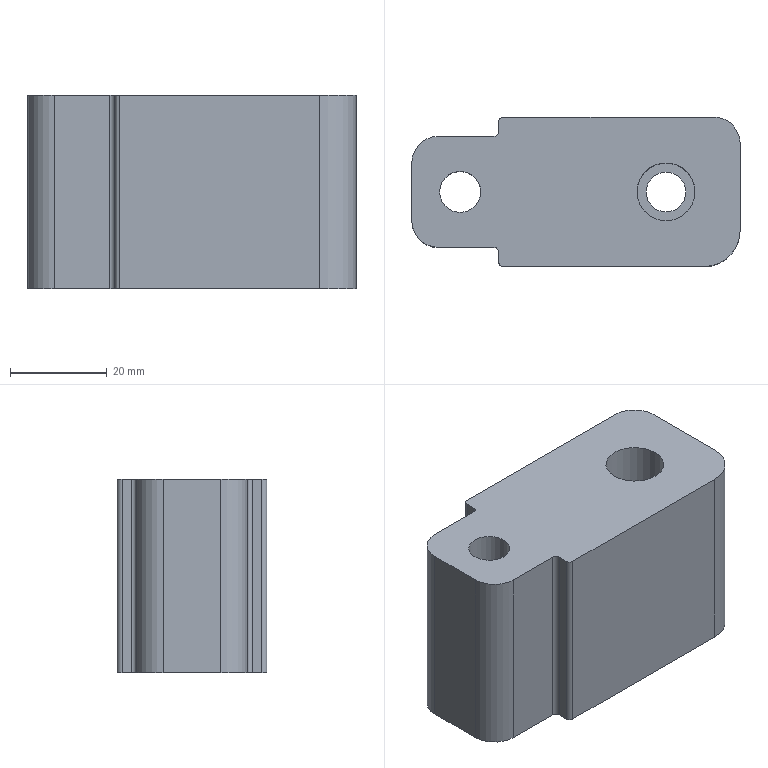Part | NX | features PS-2 2 | 1 solid | 24 faces | box 68 x 31 x 40 mm | volume 69968 mm3 | plane 12 | cylinder 12 | commonest cylinder face diameters 2 x4 11 x3 8.25 x1 8.5 x1 12 x1 14.5 x1
STEP:
#1=CARTESIAN_POINT('',(2363.049,-873.622,900.716));
#2=VERTEX_POINT('',#1);
#3=CARTESIAN_POINT('',(2404.549,-873.622,900.716));
#4=VERTEX_POINT('',#3);
#5=CARTESIAN_POINT('',(0.,-873.622,900.716));
#6=DIRECTION('',(1.,0.,0.));
#7=VECTOR('',#6,1000.);
#8=LINE('',#5,#7);
#9=EDGE_CURVE('',#2,#4,#8,.T.);
#10=ORIENTED_EDGE('',*,*,#9,.F.);
#11=CARTESIAN_POINT('',(2363.049,-873.622,860.716));
#12=VERTEX_POINT('',#11);
#13=CARTESIAN_POINT('',(2363.049,-873.622,830.716));
#14=DIRECTION('',(0.,0.,-1.));
#15=VECTOR('',#14,1000.);
#16=LINE('',#13,#15);
#17=EDGE_CURVE('',#2,#12,#16,.T.);
#18=ORIENTED_EDGE('',*,*,#17,.T.);
#19=CARTESIAN_POINT('',(2404.549,-873.622,860.716));
#20=VERTEX_POINT('',#19);
#21=CARTESIAN_POINT('',(2367.549,-873.622,860.716));
#22=DIRECTION('',(-1.,0.,0.));
#23=VECTOR('',#22,1000.);
#24=LINE('',#21,#23);
#25=EDGE_CURVE('',#20,#12,#24,.T.);
#26=ORIENTED_EDGE('',*,*,#25,.F.);
#27=CARTESIAN_POINT('',(2404.549,-873.622,830.716));
#28=DIRECTION('',(0.,0.,1.));
#29=VECTOR('',#28,1000.);
#30=LINE('',#27,#29);
#31=EDGE_CURVE('',#4,#20,#30,.F.);
#32=ORIENTED_EDGE('',*,*,#31,.F.);
#33=EDGE_LOOP('',(#10,#18,#26,#32));
#34=FACE_BOUND('',#33,.T.);
#35=CARTESIAN_POINT('',(2367.549,-873.622,830.716));
#36=DIRECTION('',(0.,-1.,0.));
#37=DIRECTION('',(0.,0.,-1.));
#38=AXIS2_PLACEMENT_3D('',#35,#36,#37);
#39=PLANE('',#38);
#40=ADVANCED_FACE('',(#34),#39,.T.);
#41=ORIENTED_EDGE('',*,*,#31,.T.);
#42=CARTESIAN_POINT('',(2412.049,-866.122,860.716));
#43=VERTEX_POINT('',#42);
#44=CARTESIAN_POINT('',(2404.549,-866.122,860.716));
#45=DIRECTION('',(0.,0.,1.));
#46=DIRECTION('',(1.,0.,0.));
#47=AXIS2_PLACEMENT_3D('',#44,#45,#46);
#48=CIRCLE('',#47,7.5);
#49=EDGE_CURVE('',#43,#20,#48,.F.);
#50=ORIENTED_EDGE('',*,*,#49,.F.);
#51=CARTESIAN_POINT('',(2412.049,-866.122,900.716));
#52=VERTEX_POINT('',#51);
#53=CARTESIAN_POINT('',(2412.049,-866.122,830.716));
#54=DIRECTION('',(0.,0.,-1.));
#55=VECTOR('',#54,1000.);
#56=LINE('',#53,#55);
#57=EDGE_CURVE('',#52,#43,#56,.T.);
#58=ORIENTED_EDGE('',*,*,#57,.F.);
#59=CARTESIAN_POINT('',(2404.549,-866.122,900.716));
#60=DIRECTION('',(0.,0.,1.));
#61=DIRECTION('',(1.,0.,0.));
#62=AXIS2_PLACEMENT_3D('',#59,#60,#61);
#63=CIRCLE('',#62,7.5);
#64=EDGE_CURVE('',#52,#4,#63,.F.);
#65=ORIENTED_EDGE('',*,*,#64,.T.);
#66=EDGE_LOOP('',(#41,#50,#58,#65));
#67=FACE_BOUND('',#66,.T.);
#68=CARTESIAN_POINT('',(2404.549,-866.122,830.716));
#69=DIRECTION('',(0.,0.,1.));
#70=DIRECTION('',(1.,0.,0.));
#71=AXIS2_PLACEMENT_3D('',#68,#69,#70);
#72=CYLINDRICAL_SURFACE('',#71,7.5);
#73=ADVANCED_FACE('',(#67),#72,.T.);
#74=ORIENTED_EDGE('',*,*,#57,.T.);
#75=CARTESIAN_POINT('',(2412.049,-848.122,860.716));
#76=VERTEX_POINT('',#75);
#77=CARTESIAN_POINT('',(2412.049,0.,860.716));
#78=DIRECTION('',(0.,1.,0.));
#79=VECTOR('',#78,1000.);
#80=LINE('',#77,#79);
#81=EDGE_CURVE('',#43,#76,#80,.T.);
#82=ORIENTED_EDGE('',*,*,#81,.T.);
#83=CARTESIAN_POINT('',(2412.049,-848.122,900.716));
#84=VERTEX_POINT('',#83);
#85=CARTESIAN_POINT('',(2412.049,-848.122,830.716));
#86=DIRECTION('',(0.,0.,1.));
#87=VECTOR('',#86,1000.);
#88=LINE('',#85,#87);
#89=EDGE_CURVE('',#84,#76,#88,.F.);
#90=ORIENTED_EDGE('',*,*,#89,.F.);
#91=CARTESIAN_POINT('',(2412.049,-866.122,900.716));
#92=DIRECTION('',(0.,-1.,0.));
#93=VECTOR('',#92,1000.);
#94=LINE('',#91,#93);
#95=EDGE_CURVE('',#84,#52,#94,.T.);
#96=ORIENTED_EDGE('',*,*,#95,.T.);
#97=EDGE_LOOP('',(#74,#82,#90,#96));
#98=FACE_BOUND('',#97,.T.);
#99=CARTESIAN_POINT('',(2412.049,-866.122,830.716));
#100=DIRECTION('',(1.,0.,0.));
#101=DIRECTION('',(0.,0.,-1.));
#102=AXIS2_PLACEMENT_3D('',#99,#100,#101);
#103=PLANE('',#102);
#104=ADVANCED_FACE('',(#98),#103,.T.);
#105=ORIENTED_EDGE('',*,*,#89,.T.);
#106=CARTESIAN_POINT('',(2406.549,-842.622,860.716));
#107=VERTEX_POINT('',#106);
#108=CARTESIAN_POINT('',(2406.549,-848.122,860.716));
#109=DIRECTION('',(0.,0.,1.));
#110=DIRECTION('',(1.,0.,0.));
#111=AXIS2_PLACEMENT_3D('',#108,#109,#110);
#112=CIRCLE('',#111,5.5);
#113=EDGE_CURVE('',#107,#76,#112,.F.);
#114=ORIENTED_EDGE('',*,*,#113,.F.);
#115=CARTESIAN_POINT('',(2406.549,-842.622,900.716));
#116=VERTEX_POINT('',#115);
#117=CARTESIAN_POINT('',(2406.549,-842.622,830.716));
#118=DIRECTION('',(0.,0.,1.));
#119=VECTOR('',#118,1000.);
#120=LINE('',#117,#119);
#121=EDGE_CURVE('',#116,#107,#120,.F.);
#122=ORIENTED_EDGE('',*,*,#121,.F.);
#123=CARTESIAN_POINT('',(2406.549,-848.122,900.716));
#124=DIRECTION('',(0.,0.,1.));
#125=DIRECTION('',(1.,0.,0.));
#126=AXIS2_PLACEMENT_3D('',#123,#124,#125);
#127=CIRCLE('',#126,5.5);
#128=EDGE_CURVE('',#84,#116,#127,.T.);
#129=ORIENTED_EDGE('',*,*,#128,.F.);
#130=EDGE_LOOP('',(#105,#114,#122,#129));
#131=FACE_BOUND('',#130,.T.);
#132=CARTESIAN_POINT('',(2406.549,-848.122,830.716));
#133=DIRECTION('',(0.,0.,1.));
#134=DIRECTION('',(1.,0.,0.));
#135=AXIS2_PLACEMENT_3D('',#132,#133,#134);
#136=CYLINDRICAL_SURFACE('',#135,5.5);
#137=ADVANCED_FACE('',(#131),#136,.T.);
#138=CARTESIAN_POINT('',(2363.049,-842.622,860.716));
#139=VERTEX_POINT('',#138);
#140=CARTESIAN_POINT('',(0.,-842.622,860.716));
#141=DIRECTION('',(-1.,0.,0.));
#142=VECTOR('',#141,1000.);
#143=LINE('',#140,#142);
#144=EDGE_CURVE('',#107,#139,#143,.T.);
#145=ORIENTED_EDGE('',*,*,#144,.T.);
#146=CARTESIAN_POINT('',(2363.049,-842.622,900.716));
#147=VERTEX_POINT('',#146);
#148=CARTESIAN_POINT('',(2363.049,-842.622,830.716));
#149=DIRECTION('',(0.,0.,1.));
#150=VECTOR('',#149,1000.);
#151=LINE('',#148,#150);
#152=EDGE_CURVE('',#139,#147,#151,.T.);
#153=ORIENTED_EDGE('',*,*,#152,.T.);
#154=CARTESIAN_POINT('',(2406.549,-842.622,900.716));
#155=DIRECTION('',(1.,0.,0.));
#156=VECTOR('',#155,1000.);
#157=LINE('',#154,#156);
#158=EDGE_CURVE('',#147,#116,#157,.T.);
#159=ORIENTED_EDGE('',*,*,#158,.T.);
#160=ORIENTED_EDGE('',*,*,#121,.T.);
#161=EDGE_LOOP('',(#145,#153,#159,#160));
#162=FACE_BOUND('',#161,.T.);
#163=CARTESIAN_POINT('',(2406.549,-842.622,830.716));
#164=DIRECTION('',(0.,1.,0.));
#165=DIRECTION('',(0.,0.,1.));
#166=AXIS2_PLACEMENT_3D('',#163,#164,#165);
#167=PLANE('',#166);
#168=ADVANCED_FACE('',(#162),#167,.T.);
#169=CARTESIAN_POINT('',(2362.049,-872.622,900.716));
#170=VERTEX_POINT('',#169);
#171=CARTESIAN_POINT('',(2362.049,-870.622,900.716));
#172=VERTEX_POINT('',#171);
#173=CARTESIAN_POINT('',(2362.049,-858.122,900.716));
#174=DIRECTION('',(0.,1.,0.));
#175=VECTOR('',#174,1000.);
#176=LINE('',#173,#175);
#177=EDGE_CURVE('',#170,#172,#176,.T.);
#178=ORIENTED_EDGE('',*,*,#177,.T.);
#179=CARTESIAN_POINT('',(2362.049,-870.622,860.716));
#180=VERTEX_POINT('',#179);
#181=CARTESIAN_POINT('',(2362.049,-870.622,860.716));
#182=DIRECTION('',(0.,0.,-1.));
#183=VECTOR('',#182,1000.);
#184=LINE('',#181,#183);
#185=EDGE_CURVE('',#172,#180,#184,.T.);
#186=ORIENTED_EDGE('',*,*,#185,.T.);
#187=CARTESIAN_POINT('',(2362.049,-872.622,860.716));
#188=VERTEX_POINT('',#187);
#189=CARTESIAN_POINT('',(2362.049,0.,860.716));
#190=DIRECTION('',(0.,-1.,0.));
#191=VECTOR('',#190,1000.);
#192=LINE('',#189,#191);
#193=EDGE_CURVE('',#180,#188,#192,.T.);
#194=ORIENTED_EDGE('',*,*,#193,.T.);
#195=CARTESIAN_POINT('',(2362.049,-872.622,875.716));
#196=DIRECTION('',(0.,0.,-1.));
#197=VECTOR('',#196,1000.);
#198=LINE('',#195,#197);
#199=EDGE_CURVE('',#188,#170,#198,.F.);
#200=ORIENTED_EDGE('',*,*,#199,.T.);
#201=EDGE_LOOP('',(#178,#186,#194,#200));
#202=FACE_BOUND('',#201,.T.);
#203=CARTESIAN_POINT('',(2362.049,-858.122,875.716));
#204=DIRECTION('',(-1.,0.,0.));
#205=DIRECTION('',(0.,0.,1.));
#206=AXIS2_PLACEMENT_3D('',#203,#204,#205);
#207=PLANE('',#206);
#208=ADVANCED_FACE('',(#202),#207,.T.);
#209=CARTESIAN_POINT('',(2362.049,-845.622,900.716));
#210=VERTEX_POINT('',#209);
#211=CARTESIAN_POINT('',(2362.049,-843.622,900.716));
#212=VERTEX_POINT('',#211);
#213=CARTESIAN_POINT('',(2362.049,-858.122,900.716));
#214=DIRECTION('',(0.,1.,0.));
#215=VECTOR('',#214,1000.);
#216=LINE('',#213,#215);
#217=EDGE_CURVE('',#210,#212,#216,.T.);
#218=ORIENTED_EDGE('',*,*,#217,.T.);
#219=CARTESIAN_POINT('',(2362.049,-843.622,860.716));
#220=VERTEX_POINT('',#219);
#221=CARTESIAN_POINT('',(2362.049,-843.622,875.716));
#222=DIRECTION('',(0.,0.,1.));
#223=VECTOR('',#222,1000.);
#224=LINE('',#221,#223);
#225=EDGE_CURVE('',#212,#220,#224,.F.);
#226=ORIENTED_EDGE('',*,*,#225,.T.);
#227=CARTESIAN_POINT('',(2362.049,-845.622,860.716));
#228=VERTEX_POINT('',#227);
#229=CARTESIAN_POINT('',(2362.049,0.,860.716));
#230=DIRECTION('',(0.,-1.,0.));
#231=VECTOR('',#230,1000.);
#232=LINE('',#229,#231);
#233=EDGE_CURVE('',#220,#228,#232,.T.);
#234=ORIENTED_EDGE('',*,*,#233,.T.);
#235=CARTESIAN_POINT('',(2362.049,-845.622,890.716));
#236=DIRECTION('',(0.,0.,1.));
#237=VECTOR('',#236,1000.);
#238=LINE('',#235,#237);
#239=EDGE_CURVE('',#228,#210,#238,.T.);
#240=ORIENTED_EDGE('',*,*,#239,.T.);
#241=EDGE_LOOP('',(#218,#226,#234,#240));
#242=FACE_BOUND('',#241,.T.);
#243=CARTESIAN_POINT('',(2362.049,-858.122,875.716));
#244=DIRECTION('',(-1.,0.,0.));
#245=DIRECTION('',(0.,0.,1.));
#246=AXIS2_PLACEMENT_3D('',#243,#244,#245);
#247=PLANE('',#246);
#248=ADVANCED_FACE('',(#242),#247,.T.);
#249=CARTESIAN_POINT('',(2344.049,-852.122,900.716));
#250=VERTEX_POINT('',#249);
#251=CARTESIAN_POINT('',(2344.049,-852.122,860.716));
#252=VERTEX_POINT('',#251);
#253=CARTESIAN_POINT('',(2344.049,-852.122,830.716));
#254=DIRECTION('',(0.,0.,1.));
#255=VECTOR('',#254,1000.);
#256=LINE('',#253,#255);
#257=EDGE_CURVE('',#250,#252,#256,.F.);
#258=ORIENTED_EDGE('',*,*,#257,.T.);
#259=CARTESIAN_POINT('',(2344.049,-864.122,860.716));
#260=VERTEX_POINT('',#259);
#261=CARTESIAN_POINT('',(2344.049,-848.122,860.716));
#262=DIRECTION('',(0.,1.,0.));
#263=VECTOR('',#262,1000.);
#264=LINE('',#261,#263);
#265=EDGE_CURVE('',#260,#252,#264,.T.);
#266=ORIENTED_EDGE('',*,*,#265,.F.);
#267=CARTESIAN_POINT('',(2344.049,-864.122,900.716));
#268=VERTEX_POINT('',#267);
#269=CARTESIAN_POINT('',(2344.049,-864.122,830.716));
#270=DIRECTION('',(0.,0.,1.));
#271=VECTOR('',#270,1000.);
#272=LINE('',#269,#271);
#273=EDGE_CURVE('',#268,#260,#272,.F.);
#274=ORIENTED_EDGE('',*,*,#273,.F.);
#275=CARTESIAN_POINT('',(2344.049,-848.122,900.716));
#276=DIRECTION('',(0.,1.,0.));
#277=VECTOR('',#276,1000.);
#278=LINE('',#275,#277);
#279=EDGE_CURVE('',#268,#250,#278,.T.);
#280=ORIENTED_EDGE('',*,*,#279,.T.);
#281=EDGE_LOOP('',(#258,#266,#274,#280));
#282=FACE_BOUND('',#281,.T.);
#283=CARTESIAN_POINT('',(2344.049,-848.122,830.716));
#284=DIRECTION('',(-1.,0.,0.));
#285=DIRECTION('',(0.,0.,1.));
#286=AXIS2_PLACEMENT_3D('',#283,#284,#285);
#287=PLANE('',#286);
#288=ADVANCED_FACE('',(#282),#287,.T.);
#289=ORIENTED_EDGE('',*,*,#273,.T.);
#290=CARTESIAN_POINT('',(2349.549,-869.622,860.716));
#291=VERTEX_POINT('',#290);
#292=CARTESIAN_POINT('',(2349.549,-864.122,860.716));
#293=DIRECTION('',(0.,0.,1.));
#294=DIRECTION('',(1.,0.,0.));
#295=AXIS2_PLACEMENT_3D('',#292,#293,#294);
#296=CIRCLE('',#295,5.5);
#297=EDGE_CURVE('',#291,#260,#296,.F.);
#298=ORIENTED_EDGE('',*,*,#297,.F.);
#299=CARTESIAN_POINT('',(2349.549,-869.622,900.716));
#300=VERTEX_POINT('',#299);
#301=CARTESIAN_POINT('',(2349.549,-869.622,830.716));
#302=DIRECTION('',(0.,0.,-1.));
#303=VECTOR('',#302,1000.);
#304=LINE('',#301,#303);
#305=EDGE_CURVE('',#300,#291,#304,.T.);
#306=ORIENTED_EDGE('',*,*,#305,.F.);
#307=CARTESIAN_POINT('',(2349.549,-864.122,900.716));
#308=DIRECTION('',(0.,0.,1.));
#309=DIRECTION('',(1.,0.,0.));
#310=AXIS2_PLACEMENT_3D('',#307,#308,#309);
#311=CIRCLE('',#310,5.5);
#312=EDGE_CURVE('',#300,#268,#311,.F.);
#313=ORIENTED_EDGE('',*,*,#312,.T.);
#314=EDGE_LOOP('',(#289,#298,#306,#313));
#315=FACE_BOUND('',#314,.T.);
#316=CARTESIAN_POINT('',(2349.549,-864.122,830.716));
#317=DIRECTION('',(0.,0.,1.));
#318=DIRECTION('',(1.,0.,0.));
#319=AXIS2_PLACEMENT_3D('',#316,#317,#318);
#320=CYLINDRICAL_SURFACE('',#319,5.5);
#321=ADVANCED_FACE('',(#315),#320,.T.);
#322=CARTESIAN_POINT('',(2361.049,-869.622,860.716));
#323=VERTEX_POINT('',#322);
#324=CARTESIAN_POINT('',(2367.549,-869.622,860.716));
#325=DIRECTION('',(-1.,0.,0.));
#326=VECTOR('',#325,1000.);
#327=LINE('',#324,#326);
#328=EDGE_CURVE('',#323,#291,#327,.T.);
#329=ORIENTED_EDGE('',*,*,#328,.F.);
#330=CARTESIAN_POINT('',(2361.049,-869.622,900.716));
#331=VERTEX_POINT('',#330);
#332=CARTESIAN_POINT('',(2361.049,-869.622,890.716));
#333=DIRECTION('',(0.,0.,-1.));
#334=VECTOR('',#333,1000.);
#335=LINE('',#332,#334);
#336=EDGE_CURVE('',#323,#331,#335,.F.);
#337=ORIENTED_EDGE('',*,*,#336,.T.);
#338=CARTESIAN_POINT('',(0.,-869.622,900.716));
#339=DIRECTION('',(1.,0.,0.));
#340=VECTOR('',#339,1000.);
#341=LINE('',#338,#340);
#342=EDGE_CURVE('',#300,#331,#341,.T.);
#343=ORIENTED_EDGE('',*,*,#342,.F.);
#344=ORIENTED_EDGE('',*,*,#305,.T.);
#345=EDGE_LOOP('',(#329,#337,#343,#344));
#346=FACE_BOUND('',#345,.T.);
#347=CARTESIAN_POINT('',(2367.549,-869.622,830.716));
#348=DIRECTION('',(0.,-1.,0.));
#349=DIRECTION('',(0.,0.,-1.));
#350=AXIS2_PLACEMENT_3D('',#347,#348,#349);
#351=PLANE('',#350);
#352=ADVANCED_FACE('',(#346),#351,.T.);
#353=CARTESIAN_POINT('',(2349.549,-846.622,900.716));
#354=VERTEX_POINT('',#353);
#355=CARTESIAN_POINT('',(2361.049,-846.622,900.716));
#356=VERTEX_POINT('',#355);
#357=CARTESIAN_POINT('',(2406.549,-846.622,900.716));
#358=DIRECTION('',(1.,0.,0.));
#359=VECTOR('',#358,1000.);
#360=LINE('',#357,#359);
#361=EDGE_CURVE('',#354,#356,#360,.T.);
#362=ORIENTED_EDGE('',*,*,#361,.T.);
#363=CARTESIAN_POINT('',(2361.049,-846.622,860.716));
#364=VERTEX_POINT('',#363);
#365=CARTESIAN_POINT('',(2361.049,-846.622,860.716));
#366=DIRECTION('',(0.,0.,1.));
#367=VECTOR('',#366,1000.);
#368=LINE('',#365,#367);
#369=EDGE_CURVE('',#356,#364,#368,.F.);
#370=ORIENTED_EDGE('',*,*,#369,.T.);
#371=CARTESIAN_POINT('',(2349.549,-846.622,860.716));
#372=VERTEX_POINT('',#371);
#373=CARTESIAN_POINT('',(0.,-846.622,860.716));
#374=DIRECTION('',(-1.,0.,0.));
#375=VECTOR('',#374,1000.);
#376=LINE('',#373,#375);
#377=EDGE_CURVE('',#364,#372,#376,.T.);
#378=ORIENTED_EDGE('',*,*,#377,.T.);
#379=CARTESIAN_POINT('',(2349.549,-846.622,830.716));
#380=DIRECTION('',(0.,0.,1.));
#381=VECTOR('',#380,1000.);
#382=LINE('',#379,#381);
#383=EDGE_CURVE('',#354,#372,#382,.F.);
#384=ORIENTED_EDGE('',*,*,#383,.F.);
#385=EDGE_LOOP('',(#362,#370,#378,#384));
#386=FACE_BOUND('',#385,.T.);
#387=CARTESIAN_POINT('',(2406.549,-846.622,830.716));
#388=DIRECTION('',(0.,1.,0.));
#389=DIRECTION('',(0.,0.,1.));
#390=AXIS2_PLACEMENT_3D('',#387,#388,#389);
#391=PLANE('',#390);
#392=ADVANCED_FACE('',(#386),#391,.T.);
#393=ORIENTED_EDGE('',*,*,#383,.T.);
#394=CARTESIAN_POINT('',(2349.549,-852.122,860.716));
#395=DIRECTION('',(0.,0.,1.));
#396=DIRECTION('',(1.,0.,0.));
#397=AXIS2_PLACEMENT_3D('',#394,#395,#396);
#398=CIRCLE('',#397,5.5);
#399=EDGE_CURVE('',#372,#252,#398,.T.);
#400=ORIENTED_EDGE('',*,*,#399,.T.);
#401=ORIENTED_EDGE('',*,*,#257,.F.);
#402=CARTESIAN_POINT('',(2349.549,-852.122,900.716));
#403=DIRECTION('',(0.,0.,1.));
#404=DIRECTION('',(1.,0.,0.));
#405=AXIS2_PLACEMENT_3D('',#402,#403,#404);
#406=CIRCLE('',#405,5.5);
#407=EDGE_CURVE('',#354,#250,#406,.T.);
#408=ORIENTED_EDGE('',*,*,#407,.F.);
#409=EDGE_LOOP('',(#393,#400,#401,#408));
#410=FACE_BOUND('',#409,.T.);
#411=CARTESIAN_POINT('',(2349.549,-852.122,830.716));
#412=DIRECTION('',(0.,0.,1.));
#413=DIRECTION('',(1.,0.,0.));
#414=AXIS2_PLACEMENT_3D('',#411,#412,#413);
#415=CYLINDRICAL_SURFACE('',#414,5.5);
#416=ADVANCED_FACE('',(#410),#415,.T.);
#417=CARTESIAN_POINT('',(2400.824,-858.122,860.716));
#418=VERTEX_POINT('',#417);
#419=CARTESIAN_POINT('',(2396.699,-858.122,860.716));
#420=DIRECTION('',(0.,0.,1.));
#421=DIRECTION('',(1.,0.,0.));
#422=AXIS2_PLACEMENT_3D('',#419,#420,#421);
#423=CIRCLE('',#422,4.125);
#424=EDGE_CURVE('',#418,#418,#423,.T.);
#425=ORIENTED_EDGE('',*,*,#424,.T.);
#426=EDGE_LOOP('',(#425));
#427=FACE_BOUND('',#426,.T.);
#428=CARTESIAN_POINT('',(2361.299,-858.122,860.716));
#429=VERTEX_POINT('',#428);
#430=CARTESIAN_POINT('',(2354.049,-858.122,860.716));
#431=DIRECTION('',(0.,0.,1.));
#432=DIRECTION('',(1.,0.,0.));
#433=AXIS2_PLACEMENT_3D('',#430,#431,#432);
#434=CIRCLE('',#433,7.25);
#435=EDGE_CURVE('',#429,#429,#434,.T.);
#436=ORIENTED_EDGE('',*,*,#435,.T.);
#437=EDGE_LOOP('',(#436));
#438=FACE_BOUND('',#437,.T.);
#439=ORIENTED_EDGE('',*,*,#233,.F.);
#440=CARTESIAN_POINT('',(2363.049,-843.622,860.716));
#441=DIRECTION('',(0.,0.,1.));
#442=DIRECTION('',(1.,0.,0.));
#443=AXIS2_PLACEMENT_3D('',#440,#441,#442);
#444=CIRCLE('',#443,1.);
#445=EDGE_CURVE('',#220,#139,#444,.F.);
#446=ORIENTED_EDGE('',*,*,#445,.T.);
#447=ORIENTED_EDGE('',*,*,#144,.F.);
#448=ORIENTED_EDGE('',*,*,#113,.T.);
#449=ORIENTED_EDGE('',*,*,#81,.F.);
#450=ORIENTED_EDGE('',*,*,#49,.T.);
#451=ORIENTED_EDGE('',*,*,#25,.T.);
#452=CARTESIAN_POINT('',(2363.049,-872.622,860.716));
#453=DIRECTION('',(0.,0.,1.));
#454=DIRECTION('',(1.,0.,0.));
#455=AXIS2_PLACEMENT_3D('',#452,#453,#454);
#456=CIRCLE('',#455,1.);
#457=EDGE_CURVE('',#12,#188,#456,.F.);
#458=ORIENTED_EDGE('',*,*,#457,.T.);
#459=ORIENTED_EDGE('',*,*,#193,.F.);
#460=CARTESIAN_POINT('',(2361.049,-870.622,860.716));
#461=DIRECTION('',(0.,0.,1.));
#462=DIRECTION('',(1.,0.,0.));
#463=AXIS2_PLACEMENT_3D('',#460,#461,#462);
#464=CIRCLE('',#463,1.);
#465=EDGE_CURVE('',#180,#323,#464,.T.);
#466=ORIENTED_EDGE('',*,*,#465,.T.);
#467=ORIENTED_EDGE('',*,*,#328,.T.);
#468=ORIENTED_EDGE('',*,*,#297,.T.);
#469=ORIENTED_EDGE('',*,*,#265,.T.);
#470=ORIENTED_EDGE('',*,*,#399,.F.);
#471=ORIENTED_EDGE('',*,*,#377,.F.);
#472=CARTESIAN_POINT('',(2361.049,-845.622,860.716));
#473=DIRECTION('',(0.,0.,1.));
#474=DIRECTION('',(1.,0.,0.));
#475=AXIS2_PLACEMENT_3D('',#472,#473,#474);
#476=CIRCLE('',#475,1.);
#477=EDGE_CURVE('',#364,#228,#476,.T.);
#478=ORIENTED_EDGE('',*,*,#477,.T.);
#479=EDGE_LOOP('',(#439,#446,#447,#448,#449,#450,#451,#458,#459,#466,#467,#468,#469,#470,#471,#478));
#480=FACE_BOUND('',#479,.T.);
#481=CARTESIAN_POINT('',(0.,0.,860.716));
#482=DIRECTION('',(0.,0.,1.));
#483=DIRECTION('',(1.,0.,0.));
#484=AXIS2_PLACEMENT_3D('',#481,#482,#483);
#485=PLANE('',#484);
#486=ADVANCED_FACE('',(#427,#438,#480),#485,.F.);
#487=CARTESIAN_POINT('',(2402.699,-858.122,900.716));
#488=VERTEX_POINT('',#487);
#489=CARTESIAN_POINT('',(2396.699,-858.122,900.716));
#490=DIRECTION('',(0.,0.,1.));
#491=DIRECTION('',(1.,0.,0.));
#492=AXIS2_PLACEMENT_3D('',#489,#490,#491);
#493=CIRCLE('',#492,6.);
#494=EDGE_CURVE('',#488,#488,#493,.T.);
#495=ORIENTED_EDGE('',*,*,#494,.F.);
#496=EDGE_LOOP('',(#495));
#497=FACE_BOUND('',#496,.T.);
#498=CARTESIAN_POINT('',(2358.299,-858.122,900.716));
#499=VERTEX_POINT('',#498);
#500=CARTESIAN_POINT('',(2354.049,-858.122,900.716));
#501=DIRECTION('',(0.,0.,1.));
#502=DIRECTION('',(1.,0.,0.));
#503=AXIS2_PLACEMENT_3D('',#500,#501,#502);
#504=CIRCLE('',#503,4.25);
#505=EDGE_CURVE('',#499,#499,#504,.T.);
#506=ORIENTED_EDGE('',*,*,#505,.F.);
#507=EDGE_LOOP('',(#506));
#508=FACE_BOUND('',#507,.T.);
#509=ORIENTED_EDGE('',*,*,#158,.F.);
#510=CARTESIAN_POINT('',(2363.049,-843.622,900.716));
#511=DIRECTION('',(0.,0.,1.));
#512=DIRECTION('',(1.,0.,0.));
#513=AXIS2_PLACEMENT_3D('',#510,#511,#512);
#514=CIRCLE('',#513,1.);
#515=EDGE_CURVE('',#147,#212,#514,.T.);
#516=ORIENTED_EDGE('',*,*,#515,.T.);
#517=ORIENTED_EDGE('',*,*,#217,.F.);
#518=CARTESIAN_POINT('',(2361.049,-845.622,900.716));
#519=DIRECTION('',(0.,0.,1.));
#520=DIRECTION('',(1.,0.,0.));
#521=AXIS2_PLACEMENT_3D('',#518,#519,#520);
#522=CIRCLE('',#521,1.);
#523=EDGE_CURVE('',#210,#356,#522,.F.);
#524=ORIENTED_EDGE('',*,*,#523,.T.);
#525=ORIENTED_EDGE('',*,*,#361,.F.);
#526=ORIENTED_EDGE('',*,*,#407,.T.);
#527=ORIENTED_EDGE('',*,*,#279,.F.);
#528=ORIENTED_EDGE('',*,*,#312,.F.);
#529=ORIENTED_EDGE('',*,*,#342,.T.);
#530=CARTESIAN_POINT('',(2361.049,-870.622,900.716));
#531=DIRECTION('',(0.,0.,1.));
#532=DIRECTION('',(1.,0.,0.));
#533=AXIS2_PLACEMENT_3D('',#530,#531,#532);
#534=CIRCLE('',#533,1.);
#535=EDGE_CURVE('',#331,#172,#534,.F.);
#536=ORIENTED_EDGE('',*,*,#535,.T.);
#537=ORIENTED_EDGE('',*,*,#177,.F.);
#538=CARTESIAN_POINT('',(2363.049,-872.622,900.716));
#539=DIRECTION('',(0.,0.,1.));
#540=DIRECTION('',(1.,0.,0.));
#541=AXIS2_PLACEMENT_3D('',#538,#539,#540);
#542=CIRCLE('',#541,1.);
#543=EDGE_CURVE('',#170,#2,#542,.T.);
#544=ORIENTED_EDGE('',*,*,#543,.T.);
#545=ORIENTED_EDGE('',*,*,#9,.T.);
#546=ORIENTED_EDGE('',*,*,#64,.F.);
#547=ORIENTED_EDGE('',*,*,#95,.F.);
#548=ORIENTED_EDGE('',*,*,#128,.T.);
#549=EDGE_LOOP('',(#509,#516,#517,#524,#525,#526,#527,#528,#529,#536,#537,#544,#545,#546,#547,#548));
#550=FACE_BOUND('',#549,.T.);
#551=CARTESIAN_POINT('',(0.,0.,900.716));
#552=DIRECTION('',(0.,0.,1.));
#553=DIRECTION('',(1.,0.,0.));
#554=AXIS2_PLACEMENT_3D('',#551,#552,#553);
#555=PLANE('',#554);
#556=ADVANCED_FACE('',(#497,#508,#550),#555,.T.);
#557=CARTESIAN_POINT('',(2354.049,-850.872,871.716));
#558=VERTEX_POINT('',#557);
#559=CARTESIAN_POINT('',(2354.049,-858.122,871.716));
#560=DIRECTION('',(0.,0.,-1.));
#561=DIRECTION('',(0.,1.,0.));
#562=AXIS2_PLACEMENT_3D('',#559,#560,#561);
#563=CIRCLE('',#562,7.25);
#564=EDGE_CURVE('',#558,#558,#563,.F.);
#565=ORIENTED_EDGE('',*,*,#564,.T.);
#566=EDGE_LOOP('',(#565));
#567=FACE_BOUND('',#566,.T.);
#568=ORIENTED_EDGE('',*,*,#435,.F.);
#569=EDGE_LOOP('',(#568));
#570=FACE_BOUND('',#569,.T.);
#571=CARTESIAN_POINT('',(2354.049,-858.122,871.716));
#572=DIRECTION('',(0.,0.,-1.));
#573=DIRECTION('',(-1.,0.,0.));
#574=AXIS2_PLACEMENT_3D('',#571,#572,#573);
#575=CYLINDRICAL_SURFACE('',#574,7.25);
#576=ADVANCED_FACE('',(#567,#570),#575,.F.);
#577=ORIENTED_EDGE('',*,*,#505,.T.);
#578=EDGE_LOOP('',(#577));
#579=FACE_BOUND('',#578,.T.);
#580=CARTESIAN_POINT('',(2349.799,-858.122,871.716));
#581=VERTEX_POINT('',#580);
#582=CARTESIAN_POINT('',(2354.049,-858.122,871.716));
#583=DIRECTION('',(0.,0.,-1.));
#584=DIRECTION('',(-1.,0.,0.));
#585=AXIS2_PLACEMENT_3D('',#582,#583,#584);
#586=CIRCLE('',#585,4.25);
#587=EDGE_CURVE('',#581,#581,#586,.T.);
#588=ORIENTED_EDGE('',*,*,#587,.T.);
#589=EDGE_LOOP('',(#588));
#590=FACE_BOUND('',#589,.T.);
#591=CARTESIAN_POINT('',(2354.049,-858.122,891.716));
#592=DIRECTION('',(0.,0.,-1.));
#593=DIRECTION('',(-1.,0.,0.));
#594=AXIS2_PLACEMENT_3D('',#591,#592,#593);
#595=CYLINDRICAL_SURFACE('',#594,4.25);
#596=ADVANCED_FACE('',(#579,#590),#595,.F.);
#597=ORIENTED_EDGE('',*,*,#587,.F.);
#598=EDGE_LOOP('',(#597));
#599=FACE_BOUND('',#598,.T.);
#600=ORIENTED_EDGE('',*,*,#564,.F.);
#601=EDGE_LOOP('',(#600));
#602=FACE_BOUND('',#601,.T.);
#603=CARTESIAN_POINT('',(2354.049,-858.122,871.716));
#604=DIRECTION('',(0.,0.,-1.));
#605=DIRECTION('',(-1.,0.,0.));
#606=AXIS2_PLACEMENT_3D('',#603,#604,#605);
#607=PLANE('',#606);
#608=ADVANCED_FACE('',(#599,#602),#607,.T.);
#609=ORIENTED_EDGE('',*,*,#445,.F.);
#610=ORIENTED_EDGE('',*,*,#225,.F.);
#611=ORIENTED_EDGE('',*,*,#515,.F.);
#612=ORIENTED_EDGE('',*,*,#152,.F.);
#613=EDGE_LOOP('',(#609,#610,#611,#612));
#614=FACE_BOUND('',#613,.T.);
#615=CARTESIAN_POINT('',(2363.049,-843.622,830.716));
#616=DIRECTION('',(0.,0.,1.));
#617=DIRECTION('',(1.,0.,0.));
#618=AXIS2_PLACEMENT_3D('',#615,#616,#617);
#619=CYLINDRICAL_SURFACE('',#618,1.);
#620=ADVANCED_FACE('',(#614),#619,.T.);
#621=ORIENTED_EDGE('',*,*,#477,.F.);
#622=ORIENTED_EDGE('',*,*,#369,.F.);
#623=ORIENTED_EDGE('',*,*,#523,.F.);
#624=ORIENTED_EDGE('',*,*,#239,.F.);
#625=EDGE_LOOP('',(#621,#622,#623,#624));
#626=FACE_BOUND('',#625,.T.);
#627=CARTESIAN_POINT('',(2361.049,-845.622,875.716));
#628=DIRECTION('',(0.,0.,-1.));
#629=DIRECTION('',(-1.,0.,0.));
#630=AXIS2_PLACEMENT_3D('',#627,#628,#629);
#631=CYLINDRICAL_SURFACE('',#630,1.);
#632=ADVANCED_FACE('',(#626),#631,.F.);
#633=ORIENTED_EDGE('',*,*,#535,.F.);
#634=ORIENTED_EDGE('',*,*,#336,.F.);
#635=ORIENTED_EDGE('',*,*,#465,.F.);
#636=ORIENTED_EDGE('',*,*,#185,.F.);
#637=EDGE_LOOP('',(#633,#634,#635,#636));
#638=FACE_BOUND('',#637,.T.);
#639=CARTESIAN_POINT('',(2361.049,-870.622,875.716));
#640=DIRECTION('',(0.,0.,1.));
#641=DIRECTION('',(1.,0.,0.));
#642=AXIS2_PLACEMENT_3D('',#639,#640,#641);
#643=CYLINDRICAL_SURFACE('',#642,1.);
#644=ADVANCED_FACE('',(#638),#643,.F.);
#645=ORIENTED_EDGE('',*,*,#543,.F.);
#646=ORIENTED_EDGE('',*,*,#199,.F.);
#647=ORIENTED_EDGE('',*,*,#457,.F.);
#648=ORIENTED_EDGE('',*,*,#17,.F.);
#649=EDGE_LOOP('',(#645,#646,#647,#648));
#650=FACE_BOUND('',#649,.T.);
#651=CARTESIAN_POINT('',(2363.049,-872.622,830.716));
#652=DIRECTION('',(0.,0.,-1.));
#653=DIRECTION('',(-1.,0.,0.));
#654=AXIS2_PLACEMENT_3D('',#651,#652,#653);
#655=CYLINDRICAL_SURFACE('',#654,1.);
#656=ADVANCED_FACE('',(#650),#655,.T.);
#657=CARTESIAN_POINT('',(2392.574,-858.122,871.716));
#658=VERTEX_POINT('',#657);
#659=CARTESIAN_POINT('',(2396.699,-858.122,871.716));
#660=DIRECTION('',(0.,0.,-1.));
#661=DIRECTION('',(-1.,0.,0.));
#662=AXIS2_PLACEMENT_3D('',#659,#660,#661);
#663=CIRCLE('',#662,4.125);
#664=EDGE_CURVE('',#658,#658,#663,.T.);
#665=ORIENTED_EDGE('',*,*,#664,.F.);
#666=EDGE_LOOP('',(#665));
#667=FACE_BOUND('',#666,.T.);
#668=ORIENTED_EDGE('',*,*,#424,.F.);
#669=EDGE_LOOP('',(#668));
#670=FACE_BOUND('',#669,.T.);
#671=CARTESIAN_POINT('',(2396.699,-858.122,935.716));
#672=DIRECTION('',(0.,0.,-1.));
#673=DIRECTION('',(1.,0.,0.));
#674=AXIS2_PLACEMENT_3D('',#671,#672,#673);
#675=CYLINDRICAL_SURFACE('',#674,4.125);
#676=ADVANCED_FACE('',(#667,#670),#675,.F.);
#677=ORIENTED_EDGE('',*,*,#664,.T.);
#678=EDGE_LOOP('',(#677));
#679=FACE_BOUND('',#678,.T.);
#680=CARTESIAN_POINT('',(2402.699,-858.122,871.716));
#681=VERTEX_POINT('',#680);
#682=CARTESIAN_POINT('',(2396.699,-858.122,871.716));
#683=DIRECTION('',(0.,0.,1.));
#684=DIRECTION('',(1.,0.,0.));
#685=AXIS2_PLACEMENT_3D('',#682,#683,#684);
#686=CIRCLE('',#685,6.);
#687=EDGE_CURVE('',#681,#681,#686,.F.);
#688=ORIENTED_EDGE('',*,*,#687,.F.);
#689=EDGE_LOOP('',(#688));
#690=FACE_BOUND('',#689,.T.);
#691=CARTESIAN_POINT('',(2396.699,-858.122,871.716));
#692=DIRECTION('',(0.,0.,-1.));
#693=DIRECTION('',(-1.,0.,0.));
#694=AXIS2_PLACEMENT_3D('',#691,#692,#693);
#695=PLANE('',#694);
#696=ADVANCED_FACE('',(#679,#690),#695,.F.);
#697=ORIENTED_EDGE('',*,*,#494,.T.);
#698=EDGE_LOOP('',(#697));
#699=FACE_BOUND('',#698,.T.);
#700=ORIENTED_EDGE('',*,*,#687,.T.);
#701=EDGE_LOOP('',(#700));
#702=FACE_BOUND('',#701,.T.);
#703=CARTESIAN_POINT('',(2396.699,-858.122,935.716));
#704=DIRECTION('',(0.,0.,-1.));
#705=DIRECTION('',(1.,0.,0.));
#706=AXIS2_PLACEMENT_3D('',#703,#704,#705);
#707=CYLINDRICAL_SURFACE('',#706,6.);
#708=ADVANCED_FACE('',(#699,#702),#707,.F.);
#709=CLOSED_SHELL('',(#40,#73,#104,#137,#168,#208,#248,#288,#321,#352,#392,#416,#486,#556,#576,#596,#608,#620,#632,#644,#656,#676,#696,#708));
#710=MANIFOLD_SOLID_BREP('',#709);
#711=(LENGTH_UNIT()NAMED_UNIT(*)SI_UNIT(.MILLI.,.METRE.));
#712=UNCERTAINTY_MEASURE_WITH_UNIT(LENGTH_MEASURE(0.00001),#711,'','');
#713=(NAMED_UNIT(*)PLANE_ANGLE_UNIT()SI_UNIT($,.RADIAN.));
#714=(NAMED_UNIT(*)SI_UNIT($,.STERADIAN.)SOLID_ANGLE_UNIT());
#715=(GEOMETRIC_REPRESENTATION_CONTEXT(3)GLOBAL_UNCERTAINTY_ASSIGNED_CONTEXT((#712))GLOBAL_UNIT_ASSIGNED_CONTEXT((#711,#713,#714))REPRESENTATION_CONTEXT('',''));
#716=ADVANCED_BREP_SHAPE_REPRESENTATION('',(#710),#715);